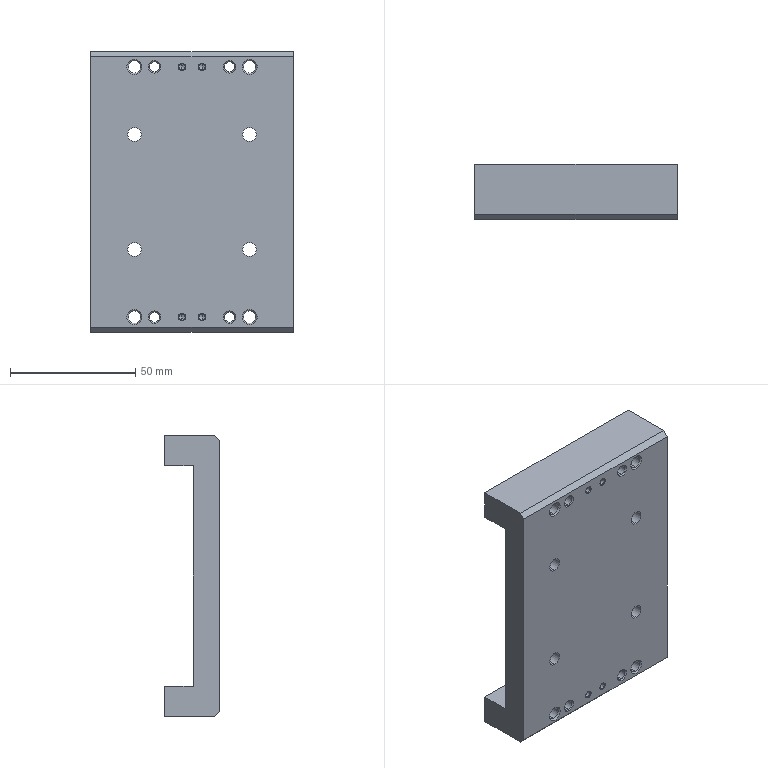Part | STEP file | 1 solid | 104 faces | box 81 x 22 x 112 mm | volume 111956 mm3 | cone 48 | cylinder 40 | plane 16 | commonest cylinder face diameters 2.459 x8 4.134 x8 4.917 x8 5.5 x8 10 x8